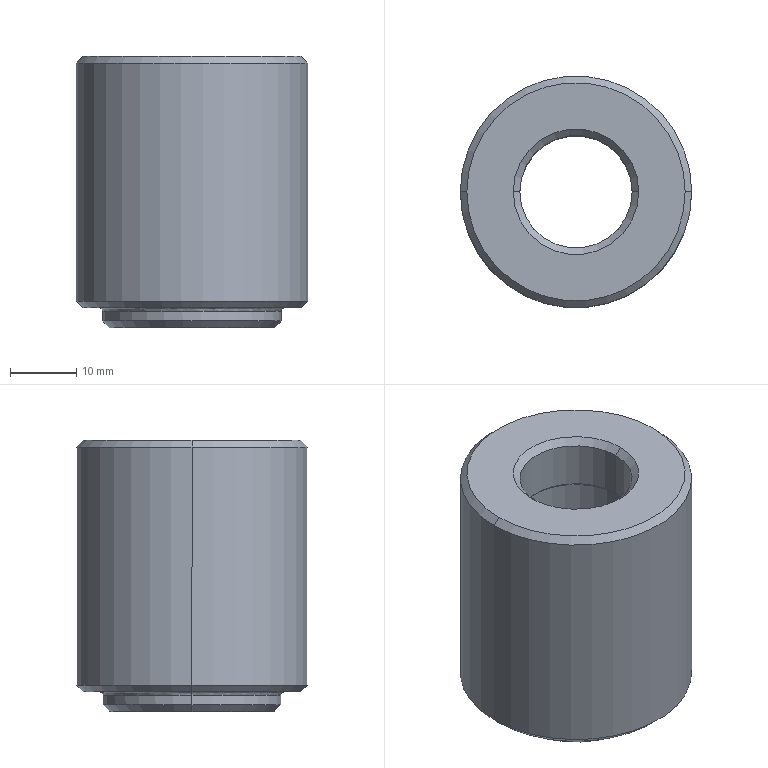Part | SolidWorks | features BaseBody 1 | 1 solid | 29 faces | box 35 x 35 x 41 mm | volume 28098 mm3 | cone 14 | cylinder 10 | plane 3 | spline 2 | commonest cylinder face diameters 17 x4 18 x2 27 x2 35 x2
STEP:
#1=CARTESIAN_POINT('',(-13.5,0.1036,-38.5));
#2=VERTEX_POINT('',#1);
#3=CARTESIAN_POINT('',(13.5,0.,-38.5));
#4=VERTEX_POINT('',#3);
#5=CARTESIAN_POINT('',(0.,0.,-38.5));
#6=DIRECTION('',(0.,0.,-1.));
#7=DIRECTION('',(1.,-0.007674,0.));
#8=AXIS2_PLACEMENT_3D('',#5,#6,#7);
#9=CIRCLE('',#8,13.5);
#10=EDGE_CURVE('',#2,#4,#9,.T.);
#11=ORIENTED_EDGE('',*,*,#10,.F.);
#12=CARTESIAN_POINT('',(-14.,0.1074,-38.));
#13=VERTEX_POINT('',#12);
#14=CARTESIAN_POINT('',(-14.,0.1074,-38.5));
#15=DIRECTION('',(-0.007674,-1.,0.));
#16=DIRECTION('',(-1.,0.007674,0.));
#17=AXIS2_PLACEMENT_3D('',#14,#15,#16);
#18=CIRCLE('',#17,0.5);
#19=EDGE_CURVE('',#2,#13,#18,.T.);
#20=ORIENTED_EDGE('',*,*,#19,.T.);
#21=CARTESIAN_POINT('',(14.,0.,-38.));
#22=VERTEX_POINT('',#21);
#23=CARTESIAN_POINT('',(-14.,0.1074,-38.));
#24=CARTESIAN_POINT('',(-13.786,27.893,-38.));
#25=CARTESIAN_POINT('',(14.,27.787,-38.));
#26=CARTESIAN_POINT('',(14.,0.,-38.));
#27=(BOUNDED_CURVE()B_SPLINE_CURVE(3,(#23,#24,#25,#26),.UNSPECIFIED.,.F.,.T.)B_SPLINE_CURVE_WITH_KNOTS((4,4),(0.002443,1.),.UNSPECIFIED.)CURVE()GEOMETRIC_REPRESENTATION_ITEM()RATIONAL_B_SPLINE_CURVE((1.,0.3359,0.3359,1.))REPRESENTATION_ITEM(''));
#28=EDGE_CURVE('',#13,#22,#27,.T.);
#29=ORIENTED_EDGE('',*,*,#28,.T.);
#30=CARTESIAN_POINT('',(14.,-0.1074,-38.));
#31=VERTEX_POINT('',#30);
#32=CARTESIAN_POINT('',(14.,0.,-38.));
#33=CARTESIAN_POINT('',(14.,-0.03581,-38.));
#34=CARTESIAN_POINT('',(14.,-0.07162,-38.));
#35=CARTESIAN_POINT('',(14.,-0.1074,-38.));
#36=(BOUNDED_CURVE()B_SPLINE_CURVE(3,(#32,#33,#34,#35),.UNSPECIFIED.,.F.,.F.)B_SPLINE_CURVE_WITH_KNOTS((4,4),(0.,0.002443),.UNSPECIFIED.)CURVE()GEOMETRIC_REPRESENTATION_ITEM()RATIONAL_B_SPLINE_CURVE((1.,1.,1.,1.))REPRESENTATION_ITEM(''));
#37=EDGE_CURVE('',#22,#31,#36,.T.);
#38=ORIENTED_EDGE('',*,*,#37,.T.);
#39=CARTESIAN_POINT('',(13.5,-0.1036,-38.5));
#40=VERTEX_POINT('',#39);
#41=CARTESIAN_POINT('',(14.,-0.1074,-38.5));
#42=DIRECTION('',(0.007674,1.,0.));
#43=DIRECTION('',(1.,-0.007674,0.));
#44=AXIS2_PLACEMENT_3D('',#41,#42,#43);
#45=CIRCLE('',#44,0.5);
#46=EDGE_CURVE('',#40,#31,#45,.T.);
#47=ORIENTED_EDGE('',*,*,#46,.F.);
#48=CARTESIAN_POINT('',(0.,0.,-38.5));
#49=DIRECTION('',(0.,0.,-1.));
#50=DIRECTION('',(1.,-0.007674,0.));
#51=AXIS2_PLACEMENT_3D('',#48,#49,#50);
#52=CIRCLE('',#51,13.5);
#53=EDGE_CURVE('',#4,#40,#52,.T.);
#54=ORIENTED_EDGE('',*,*,#53,.F.);
#55=EDGE_LOOP('',(#11,#20,#29,#38,#47,#54));
#56=FACE_OUTER_BOUND('',#55,.T.);
#57=CARTESIAN_POINT('',(13.5,-0.1036,-38.5));
#58=CARTESIAN_POINT('',(13.707,26.896,-38.5));
#59=CARTESIAN_POINT('',(-13.292,27.103,-38.5));
#60=CARTESIAN_POINT('',(-13.5,0.1036,-38.5));
#61=CARTESIAN_POINT('',(13.5,-0.1036,-38.207));
#62=CARTESIAN_POINT('',(13.707,26.896,-38.207));
#63=CARTESIAN_POINT('',(-13.292,27.103,-38.207));
#64=CARTESIAN_POINT('',(-13.5,0.1036,-38.207));
#65=CARTESIAN_POINT('',(13.707,-0.1052,-38.));
#66=CARTESIAN_POINT('',(13.917,27.308,-38.));
#67=CARTESIAN_POINT('',(-13.496,27.519,-38.));
#68=CARTESIAN_POINT('',(-13.707,0.1052,-38.));
#69=CARTESIAN_POINT('',(14.,-0.1074,-38.));
#70=CARTESIAN_POINT('',(14.214,27.892,-38.));
#71=CARTESIAN_POINT('',(-13.785,28.107,-38.));
#72=CARTESIAN_POINT('',(-14.,0.1074,-38.));
#73=(BOUNDED_SURFACE()B_SPLINE_SURFACE(3,3,((#57,#58,#59,#60),(#61,#62,#63,#64),(#65,#66,#67,#68),(#69,#70,#71,#72)),.UNSPECIFIED.,.F.,.F.,.F.)B_SPLINE_SURFACE_WITH_KNOTS((4,4),(4,4),(0.,1.),(0.,1.),.UNSPECIFIED.)GEOMETRIC_REPRESENTATION_ITEM()RATIONAL_B_SPLINE_SURFACE(((1.,0.3333,0.3333,1.),(0.8047,0.2682,0.2682,0.8047),(0.8047,0.2682,0.2682,0.8047),(1.,0.3333,0.3333,1.)))REPRESENTATION_ITEM('')SURFACE());
#74=ADVANCED_FACE('',(#56),#73,.F.);
#75=CARTESIAN_POINT('',(17.5,0.,-37.));
#76=VERTEX_POINT('',#75);
#77=CARTESIAN_POINT('',(-17.5,0.,-37.));
#78=VERTEX_POINT('',#77);
#79=CARTESIAN_POINT('',(0.,0.,-37.));
#80=DIRECTION('',(0.,0.,1.));
#81=DIRECTION('',(1.,0.,0.));
#82=AXIS2_PLACEMENT_3D('',#79,#80,#81);
#83=CIRCLE('',#82,17.5);
#84=EDGE_CURVE('',#76,#78,#83,.T.);
#85=ORIENTED_EDGE('',*,*,#84,.T.);
#86=CARTESIAN_POINT('',(-17.5,0.,-1.));
#87=VERTEX_POINT('',#86);
#88=CARTESIAN_POINT('',(-17.5,0.,-43.05));
#89=DIRECTION('',(0.,0.,1.));
#90=VECTOR('',#89,1000.);
#91=LINE('',#88,#90);
#92=EDGE_CURVE('',#78,#87,#91,.T.);
#93=ORIENTED_EDGE('',*,*,#92,.T.);
#94=CARTESIAN_POINT('',(17.5,0.,-1.));
#95=VERTEX_POINT('',#94);
#96=CARTESIAN_POINT('',(0.,0.,-1.));
#97=DIRECTION('',(0.,0.,-1.));
#98=DIRECTION('',(1.,0.,0.));
#99=AXIS2_PLACEMENT_3D('',#96,#97,#98);
#100=CIRCLE('',#99,17.5);
#101=EDGE_CURVE('',#87,#95,#100,.T.);
#102=ORIENTED_EDGE('',*,*,#101,.T.);
#103=CARTESIAN_POINT('',(17.5,0.,-43.05));
#104=DIRECTION('',(0.,0.,1.));
#105=VECTOR('',#104,1000.);
#106=LINE('',#103,#105);
#107=EDGE_CURVE('',#76,#95,#106,.T.);
#108=ORIENTED_EDGE('',*,*,#107,.F.);
#109=EDGE_LOOP('',(#85,#93,#102,#108));
#110=FACE_OUTER_BOUND('',#109,.T.);
#111=CARTESIAN_POINT('',(0.,0.,-43.05));
#112=DIRECTION('',(0.,0.,1.));
#113=DIRECTION('',(1.,0.,0.));
#114=AXIS2_PLACEMENT_3D('',#111,#112,#113);
#115=CYLINDRICAL_SURFACE('',#114,17.5);
#116=ADVANCED_FACE('',(#110),#115,.T.);
#117=CARTESIAN_POINT('',(16.5,0.,-38.));
#118=VERTEX_POINT('',#117);
#119=CARTESIAN_POINT('',(-16.5,0.,-38.));
#120=VERTEX_POINT('',#119);
#121=CARTESIAN_POINT('',(0.,0.,-38.));
#122=DIRECTION('',(0.,0.,1.));
#123=DIRECTION('',(1.,0.,0.));
#124=AXIS2_PLACEMENT_3D('',#121,#122,#123);
#125=CIRCLE('',#124,16.5);
#126=EDGE_CURVE('',#118,#120,#125,.T.);
#127=ORIENTED_EDGE('',*,*,#126,.T.);
#128=CARTESIAN_POINT('',(-17.5,0.,-37.));
#129=DIRECTION('',(-0.7071,0.,0.7071));
#130=VECTOR('',#129,1000.);
#131=LINE('',#128,#130);
#132=EDGE_CURVE('',#120,#78,#131,.T.);
#133=ORIENTED_EDGE('',*,*,#132,.T.);
#134=ORIENTED_EDGE('',*,*,#84,.F.);
#135=CARTESIAN_POINT('',(17.5,0.,-37.));
#136=DIRECTION('',(0.7071,0.,0.7071));
#137=VECTOR('',#136,1000.);
#138=LINE('',#135,#137);
#139=EDGE_CURVE('',#118,#76,#138,.T.);
#140=ORIENTED_EDGE('',*,*,#139,.F.);
#141=EDGE_LOOP('',(#127,#133,#134,#140));
#142=FACE_OUTER_BOUND('',#141,.T.);
#143=CARTESIAN_POINT('',(0.,0.,-37.));
#144=DIRECTION('',(0.,0.,1.));
#145=DIRECTION('',(1.,0.,0.));
#146=AXIS2_PLACEMENT_3D('',#143,#144,#145);
#147=CONICAL_SURFACE('',#146,17.5,0.7854);
#148=ADVANCED_FACE('',(#142),#147,.T.);
#149=CARTESIAN_POINT('',(-16.5,0.,0.));
#150=VERTEX_POINT('',#149);
#151=CARTESIAN_POINT('',(16.5,0.,0.));
#152=VERTEX_POINT('',#151);
#153=CARTESIAN_POINT('',(0.,0.,0.));
#154=DIRECTION('',(0.,0.,-1.));
#155=DIRECTION('',(-1.,0.,0.));
#156=AXIS2_PLACEMENT_3D('',#153,#154,#155);
#157=CIRCLE('',#156,16.5);
#158=EDGE_CURVE('',#150,#152,#157,.T.);
#159=ORIENTED_EDGE('',*,*,#158,.T.);
#160=CARTESIAN_POINT('',(17.5,0.,-1.));
#161=DIRECTION('',(0.7071,0.,-0.7071));
#162=VECTOR('',#161,1000.);
#163=LINE('',#160,#162);
#164=EDGE_CURVE('',#152,#95,#163,.T.);
#165=ORIENTED_EDGE('',*,*,#164,.T.);
#166=ORIENTED_EDGE('',*,*,#101,.F.);
#167=CARTESIAN_POINT('',(-17.5,0.,-1.));
#168=DIRECTION('',(-0.7071,0.,-0.7071));
#169=VECTOR('',#168,1000.);
#170=LINE('',#167,#169);
#171=EDGE_CURVE('',#150,#87,#170,.T.);
#172=ORIENTED_EDGE('',*,*,#171,.F.);
#173=EDGE_LOOP('',(#159,#165,#166,#172));
#174=FACE_OUTER_BOUND('',#173,.T.);
#175=CARTESIAN_POINT('',(0.,0.,-1.));
#176=DIRECTION('',(0.,0.,-1.));
#177=DIRECTION('',(-1.,0.,0.));
#178=AXIS2_PLACEMENT_3D('',#175,#176,#177);
#179=CONICAL_SURFACE('',#178,17.5,0.7854);
#180=ADVANCED_FACE('',(#174),#179,.T.);
#181=CARTESIAN_POINT('',(-8.5,0.,-1.));
#182=VERTEX_POINT('',#181);
#183=CARTESIAN_POINT('',(8.5,0.,-1.));
#184=VERTEX_POINT('',#183);
#185=CARTESIAN_POINT('',(0.,0.,-1.));
#186=DIRECTION('',(0.,0.,1.));
#187=DIRECTION('',(0.,-1.,0.));
#188=AXIS2_PLACEMENT_3D('',#185,#186,#187);
#189=CIRCLE('',#188,8.5);
#190=EDGE_CURVE('',#182,#184,#189,.T.);
#191=ORIENTED_EDGE('',*,*,#190,.F.);
#192=CARTESIAN_POINT('',(-9.5,0.,0.));
#193=VERTEX_POINT('',#192);
#194=CARTESIAN_POINT('',(-9.5,0.,0.));
#195=DIRECTION('',(-0.7071,0.,0.7071));
#196=VECTOR('',#195,1000.);
#197=LINE('',#194,#196);
#198=EDGE_CURVE('',#182,#193,#197,.T.);
#199=ORIENTED_EDGE('',*,*,#198,.T.);
#200=CARTESIAN_POINT('',(9.5,0.,0.));
#201=VERTEX_POINT('',#200);
#202=CARTESIAN_POINT('',(0.,0.,0.));
#203=DIRECTION('',(0.,0.,-1.));
#204=DIRECTION('',(1.,0.,0.));
#205=AXIS2_PLACEMENT_3D('',#202,#203,#204);
#206=CIRCLE('',#205,9.5);
#207=EDGE_CURVE('',#201,#193,#206,.T.);
#208=ORIENTED_EDGE('',*,*,#207,.F.);
#209=CARTESIAN_POINT('',(9.5,0.,0.));
#210=DIRECTION('',(0.7071,0.,0.7071));
#211=VECTOR('',#210,1000.);
#212=LINE('',#209,#211);
#213=EDGE_CURVE('',#184,#201,#212,.T.);
#214=ORIENTED_EDGE('',*,*,#213,.F.);
#215=EDGE_LOOP('',(#191,#199,#208,#214));
#216=FACE_OUTER_BOUND('',#215,.T.);
#217=CARTESIAN_POINT('',(0.,0.,0.));
#218=DIRECTION('',(0.,0.,1.));
#219=DIRECTION('',(1.,0.,0.));
#220=AXIS2_PLACEMENT_3D('',#217,#218,#219);
#221=CONICAL_SURFACE('',#220,9.5,0.7854);
#222=ADVANCED_FACE('',(#216),#221,.F.);
#223=CARTESIAN_POINT('',(13.5,0.,-40.));
#224=VERTEX_POINT('',#223);
#225=CARTESIAN_POINT('',(-13.5,0.,-40.));
#226=VERTEX_POINT('',#225);
#227=CARTESIAN_POINT('',(0.,0.,-40.));
#228=DIRECTION('',(0.,0.,1.));
#229=DIRECTION('',(1.,0.,0.));
#230=AXIS2_PLACEMENT_3D('',#227,#228,#229);
#231=CIRCLE('',#230,13.5);
#232=EDGE_CURVE('',#224,#226,#231,.T.);
#233=ORIENTED_EDGE('',*,*,#232,.T.);
#234=CARTESIAN_POINT('',(-13.5,0.,-38.5));
#235=VERTEX_POINT('',#234);
#236=CARTESIAN_POINT('',(-13.5,0.,-43.05));
#237=DIRECTION('',(0.,0.,1.));
#238=VECTOR('',#237,1000.);
#239=LINE('',#236,#238);
#240=EDGE_CURVE('',#226,#235,#239,.T.);
#241=ORIENTED_EDGE('',*,*,#240,.T.);
#242=CARTESIAN_POINT('',(0.,0.,-38.5));
#243=DIRECTION('',(0.,0.,-1.));
#244=DIRECTION('',(1.,-0.007674,0.));
#245=AXIS2_PLACEMENT_3D('',#242,#243,#244);
#246=CIRCLE('',#245,13.5);
#247=EDGE_CURVE('',#235,#2,#246,.T.);
#248=ORIENTED_EDGE('',*,*,#247,.T.);
#249=ORIENTED_EDGE('',*,*,#10,.T.);
#250=CARTESIAN_POINT('',(13.5,0.,-43.05));
#251=DIRECTION('',(0.,0.,1.));
#252=VECTOR('',#251,1000.);
#253=LINE('',#250,#252);
#254=EDGE_CURVE('',#224,#4,#253,.T.);
#255=ORIENTED_EDGE('',*,*,#254,.F.);
#256=EDGE_LOOP('',(#233,#241,#248,#249,#255));
#257=FACE_OUTER_BOUND('',#256,.T.);
#258=CARTESIAN_POINT('',(0.,0.,-43.05));
#259=DIRECTION('',(0.,0.,1.));
#260=DIRECTION('',(1.,0.,0.));
#261=AXIS2_PLACEMENT_3D('',#258,#259,#260);
#262=CYLINDRICAL_SURFACE('',#261,13.5);
#263=ADVANCED_FACE('',(#257),#262,.T.);
#264=CARTESIAN_POINT('',(-8.5,0.,-8.));
#265=VERTEX_POINT('',#264);
#266=CARTESIAN_POINT('',(8.5,0.,-8.));
#267=VERTEX_POINT('',#266);
#268=CARTESIAN_POINT('',(0.,0.,-8.));
#269=DIRECTION('',(0.,0.,1.));
#270=DIRECTION('',(1.,0.,0.));
#271=AXIS2_PLACEMENT_3D('',#268,#269,#270);
#272=CIRCLE('',#271,8.5);
#273=EDGE_CURVE('',#265,#267,#272,.T.);
#274=ORIENTED_EDGE('',*,*,#273,.F.);
#275=CARTESIAN_POINT('',(-8.5,0.,-43.05));
#276=DIRECTION('',(0.,0.,1.));
#277=VECTOR('',#276,1000.);
#278=LINE('',#275,#277);
#279=EDGE_CURVE('',#265,#182,#278,.T.);
#280=ORIENTED_EDGE('',*,*,#279,.T.);
#281=ORIENTED_EDGE('',*,*,#190,.T.);
#282=CARTESIAN_POINT('',(8.5,0.,-43.05));
#283=DIRECTION('',(0.,0.,1.));
#284=VECTOR('',#283,1000.);
#285=LINE('',#282,#284);
#286=EDGE_CURVE('',#267,#184,#285,.T.);
#287=ORIENTED_EDGE('',*,*,#286,.F.);
#288=EDGE_LOOP('',(#274,#280,#281,#287));
#289=FACE_OUTER_BOUND('',#288,.T.);
#290=CARTESIAN_POINT('',(0.,0.,-43.05));
#291=DIRECTION('',(0.,0.,1.));
#292=DIRECTION('',(1.,0.,0.));
#293=AXIS2_PLACEMENT_3D('',#290,#291,#292);
#294=CYLINDRICAL_SURFACE('',#293,8.5);
#295=ADVANCED_FACE('',(#289),#294,.F.);
#296=CARTESIAN_POINT('',(12.5,0.,-41.));
#297=VERTEX_POINT('',#296);
#298=CARTESIAN_POINT('',(-12.5,0.,-41.));
#299=VERTEX_POINT('',#298);
#300=CARTESIAN_POINT('',(0.,0.,-41.));
#301=DIRECTION('',(0.,0.,1.));
#302=DIRECTION('',(1.,0.,0.));
#303=AXIS2_PLACEMENT_3D('',#300,#301,#302);
#304=CIRCLE('',#303,12.5);
#305=EDGE_CURVE('',#297,#299,#304,.T.);
#306=ORIENTED_EDGE('',*,*,#305,.T.);
#307=CARTESIAN_POINT('',(-13.5,0.,-40.));
#308=DIRECTION('',(-0.7071,0.,0.7071));
#309=VECTOR('',#308,1000.);
#310=LINE('',#307,#309);
#311=EDGE_CURVE('',#299,#226,#310,.T.);
#312=ORIENTED_EDGE('',*,*,#311,.T.);
#313=ORIENTED_EDGE('',*,*,#232,.F.);
#314=CARTESIAN_POINT('',(13.5,0.,-40.));
#315=DIRECTION('',(0.7071,0.,0.7071));
#316=VECTOR('',#315,1000.);
#317=LINE('',#314,#316);
#318=EDGE_CURVE('',#297,#224,#317,.T.);
#319=ORIENTED_EDGE('',*,*,#318,.F.);
#320=EDGE_LOOP('',(#306,#312,#313,#319));
#321=FACE_OUTER_BOUND('',#320,.T.);
#322=CARTESIAN_POINT('',(0.,0.,-40.));
#323=DIRECTION('',(0.,0.,1.));
#324=DIRECTION('',(1.,0.,0.));
#325=AXIS2_PLACEMENT_3D('',#322,#323,#324);
#326=CONICAL_SURFACE('',#325,13.5,0.7854);
#327=ADVANCED_FACE('',(#321),#326,.T.);
#328=ORIENTED_EDGE('',*,*,#273,.T.);
#329=CARTESIAN_POINT('',(9.,0.,-8.5));
#330=VERTEX_POINT('',#329);
#331=CARTESIAN_POINT('',(9.,0.,-8.5));
#332=DIRECTION('',(0.7071,0.,-0.7071));
#333=VECTOR('',#332,1000.);
#334=LINE('',#331,#333);
#335=EDGE_CURVE('',#267,#330,#334,.T.);
#336=ORIENTED_EDGE('',*,*,#335,.T.);
#337=CARTESIAN_POINT('',(-9.,0.,-8.5));
#338=VERTEX_POINT('',#337);
#339=CARTESIAN_POINT('',(0.,0.,-8.5));
#340=DIRECTION('',(0.,0.,1.));
#341=DIRECTION('',(1.,0.,0.));
#342=AXIS2_PLACEMENT_3D('',#339,#340,#341);
#343=CIRCLE('',#342,9.);
#344=EDGE_CURVE('',#338,#330,#343,.T.);
#345=ORIENTED_EDGE('',*,*,#344,.F.);
#346=CARTESIAN_POINT('',(-9.,0.,-8.5));
#347=DIRECTION('',(-0.7071,0.,-0.7071));
#348=VECTOR('',#347,1000.);
#349=LINE('',#346,#348);
#350=EDGE_CURVE('',#265,#338,#349,.T.);
#351=ORIENTED_EDGE('',*,*,#350,.F.);
#352=EDGE_LOOP('',(#328,#336,#345,#351));
#353=FACE_OUTER_BOUND('',#352,.T.);
#354=CARTESIAN_POINT('',(0.,0.,-8.5));
#355=DIRECTION('',(0.,0.,-1.));
#356=DIRECTION('',(-1.,0.,0.));
#357=AXIS2_PLACEMENT_3D('',#354,#355,#356);
#358=CONICAL_SURFACE('',#357,9.,0.7854);
#359=ADVANCED_FACE('',(#353),#358,.F.);
#360=CARTESIAN_POINT('',(-9.,0.,-32.5));
#361=VERTEX_POINT('',#360);
#362=CARTESIAN_POINT('',(9.,0.,-32.5));
#363=VERTEX_POINT('',#362);
#364=CARTESIAN_POINT('',(0.,0.,-32.5));
#365=DIRECTION('',(0.,0.,1.));
#366=DIRECTION('',(1.,0.,0.));
#367=AXIS2_PLACEMENT_3D('',#364,#365,#366);
#368=CIRCLE('',#367,9.);
#369=EDGE_CURVE('',#361,#363,#368,.T.);
#370=ORIENTED_EDGE('',*,*,#369,.F.);
#371=CARTESIAN_POINT('',(-9.,0.,-43.05));
#372=DIRECTION('',(0.,0.,1.));
#373=VECTOR('',#372,1000.);
#374=LINE('',#371,#373);
#375=EDGE_CURVE('',#361,#338,#374,.T.);
#376=ORIENTED_EDGE('',*,*,#375,.T.);
#377=ORIENTED_EDGE('',*,*,#344,.T.);
#378=CARTESIAN_POINT('',(9.,0.,-43.05));
#379=DIRECTION('',(0.,0.,1.));
#380=VECTOR('',#379,1000.);
#381=LINE('',#378,#380);
#382=EDGE_CURVE('',#363,#330,#381,.T.);
#383=ORIENTED_EDGE('',*,*,#382,.F.);
#384=EDGE_LOOP('',(#370,#376,#377,#383));
#385=FACE_OUTER_BOUND('',#384,.T.);
#386=CARTESIAN_POINT('',(0.,0.,-43.05));
#387=DIRECTION('',(0.,0.,1.));
#388=DIRECTION('',(1.,0.,0.));
#389=AXIS2_PLACEMENT_3D('',#386,#387,#388);
#390=CYLINDRICAL_SURFACE('',#389,9.);
#391=ADVANCED_FACE('',(#385),#390,.F.);
#392=CARTESIAN_POINT('',(8.5,0.,-40.));
#393=VERTEX_POINT('',#392);
#394=CARTESIAN_POINT('',(-8.5,0.,-40.));
#395=VERTEX_POINT('',#394);
#396=CARTESIAN_POINT('',(0.,0.,-40.));
#397=DIRECTION('',(0.,0.,-1.));
#398=DIRECTION('',(0.,-1.,0.));
#399=AXIS2_PLACEMENT_3D('',#396,#397,#398);
#400=CIRCLE('',#399,8.5);
#401=EDGE_CURVE('',#393,#395,#400,.T.);
#402=ORIENTED_EDGE('',*,*,#401,.F.);
#403=CARTESIAN_POINT('',(9.5,0.,-41.));
#404=VERTEX_POINT('',#403);
#405=CARTESIAN_POINT('',(9.5,0.,-41.));
#406=DIRECTION('',(0.7071,0.,-0.7071));
#407=VECTOR('',#406,1000.);
#408=LINE('',#405,#407);
#409=EDGE_CURVE('',#393,#404,#408,.T.);
#410=ORIENTED_EDGE('',*,*,#409,.T.);
#411=CARTESIAN_POINT('',(-9.5,0.,-41.));
#412=VERTEX_POINT('',#411);
#413=CARTESIAN_POINT('',(0.,0.,-41.));
#414=DIRECTION('',(0.,0.,-1.));
#415=DIRECTION('',(-1.,0.,0.));
#416=AXIS2_PLACEMENT_3D('',#413,#414,#415);
#417=CIRCLE('',#416,9.5);
#418=EDGE_CURVE('',#404,#412,#417,.T.);
#419=ORIENTED_EDGE('',*,*,#418,.T.);
#420=CARTESIAN_POINT('',(-9.5,0.,-41.));
#421=DIRECTION('',(-0.7071,0.,-0.7071));
#422=VECTOR('',#421,1000.);
#423=LINE('',#420,#422);
#424=EDGE_CURVE('',#395,#412,#423,.T.);
#425=ORIENTED_EDGE('',*,*,#424,.F.);
#426=EDGE_LOOP('',(#402,#410,#419,#425));
#427=FACE_OUTER_BOUND('',#426,.T.);
#428=CARTESIAN_POINT('',(0.,0.,-41.));
#429=DIRECTION('',(0.,0.,-1.));
#430=DIRECTION('',(-1.,0.,0.));
#431=AXIS2_PLACEMENT_3D('',#428,#429,#430);
#432=CONICAL_SURFACE('',#431,9.5,0.7854);
#433=ADVANCED_FACE('',(#427),#432,.F.);
#434=CARTESIAN_POINT('',(-8.5,0.,-33.));
#435=VERTEX_POINT('',#434);
#436=CARTESIAN_POINT('',(8.5,0.,-33.));
#437=VERTEX_POINT('',#436);
#438=CARTESIAN_POINT('',(0.,0.,-33.));
#439=DIRECTION('',(0.,0.,1.));
#440=DIRECTION('',(-1.,0.,0.));
#441=AXIS2_PLACEMENT_3D('',#438,#439,#440);
#442=CIRCLE('',#441,8.5);
#443=EDGE_CURVE('',#435,#437,#442,.T.);
#444=ORIENTED_EDGE('',*,*,#443,.F.);
#445=CARTESIAN_POINT('',(-9.,0.,-32.5));
#446=DIRECTION('',(-0.7071,0.,0.7071));
#447=VECTOR('',#446,1000.);
#448=LINE('',#445,#447);
#449=EDGE_CURVE('',#435,#361,#448,.T.);
#450=ORIENTED_EDGE('',*,*,#449,.T.);
#451=ORIENTED_EDGE('',*,*,#369,.T.);
#452=CARTESIAN_POINT('',(9.,0.,-32.5));
#453=DIRECTION('',(0.7071,0.,0.7071));
#454=VECTOR('',#453,1000.);
#455=LINE('',#452,#454);
#456=EDGE_CURVE('',#437,#363,#455,.T.);
#457=ORIENTED_EDGE('',*,*,#456,.F.);
#458=EDGE_LOOP('',(#444,#450,#451,#457));
#459=FACE_OUTER_BOUND('',#458,.T.);
#460=CARTESIAN_POINT('',(0.,0.,-32.5));
#461=DIRECTION('',(0.,0.,1.));
#462=DIRECTION('',(1.,0.,0.));
#463=AXIS2_PLACEMENT_3D('',#460,#461,#462);
#464=CONICAL_SURFACE('',#463,9.,0.7854);
#465=ADVANCED_FACE('',(#459),#464,.F.);
#466=ORIENTED_EDGE('',*,*,#401,.T.);
#467=CARTESIAN_POINT('',(-8.5,0.,-43.05));
#468=DIRECTION('',(0.,0.,1.));
#469=VECTOR('',#468,1000.);
#470=LINE('',#467,#469);
#471=EDGE_CURVE('',#395,#435,#470,.T.);
#472=ORIENTED_EDGE('',*,*,#471,.T.);
#473=ORIENTED_EDGE('',*,*,#443,.T.);
#474=CARTESIAN_POINT('',(8.5,0.,-43.05));
#475=DIRECTION('',(0.,0.,1.));
#476=VECTOR('',#475,1000.);
#477=LINE('',#474,#476);
#478=EDGE_CURVE('',#393,#437,#477,.T.);
#479=ORIENTED_EDGE('',*,*,#478,.F.);
#480=EDGE_LOOP('',(#466,#472,#473,#479));
#481=FACE_OUTER_BOUND('',#480,.T.);
#482=CARTESIAN_POINT('',(0.,0.,-43.05));
#483=DIRECTION('',(0.,0.,1.));
#484=DIRECTION('',(1.,0.,0.));
#485=AXIS2_PLACEMENT_3D('',#482,#483,#484);
#486=CYLINDRICAL_SURFACE('',#485,8.5);
#487=ADVANCED_FACE('',(#481),#486,.F.);
#488=ORIENTED_EDGE('',*,*,#92,.F.);
#489=CARTESIAN_POINT('',(0.,0.,-37.));
#490=DIRECTION('',(0.,0.,1.));
#491=DIRECTION('',(1.,0.,0.));
#492=AXIS2_PLACEMENT_3D('',#489,#490,#491);
#493=CIRCLE('',#492,17.5);
#494=EDGE_CURVE('',#78,#76,#493,.T.);
#495=ORIENTED_EDGE('',*,*,#494,.T.);
#496=ORIENTED_EDGE('',*,*,#107,.T.);
#497=CARTESIAN_POINT('',(0.,0.,-1.));
#498=DIRECTION('',(0.,0.,-1.));
#499=DIRECTION('',(1.,0.,0.));
#500=AXIS2_PLACEMENT_3D('',#497,#498,#499);
#501=CIRCLE('',#500,17.5);
#502=EDGE_CURVE('',#95,#87,#501,.T.);
#503=ORIENTED_EDGE('',*,*,#502,.T.);
#504=EDGE_LOOP('',(#488,#495,#496,#503));
#505=FACE_OUTER_BOUND('',#504,.T.);
#506=CARTESIAN_POINT('',(0.,0.,-43.05));
#507=DIRECTION('',(0.,0.,1.));
#508=DIRECTION('',(1.,0.,0.));
#509=AXIS2_PLACEMENT_3D('',#506,#507,#508);
#510=CYLINDRICAL_SURFACE('',#509,17.5);
#511=ADVANCED_FACE('',(#505),#510,.T.);
#512=ORIENTED_EDGE('',*,*,#132,.F.);
#513=CARTESIAN_POINT('',(0.,0.,-38.));
#514=DIRECTION('',(0.,0.,1.));
#515=DIRECTION('',(1.,0.,0.));
#516=AXIS2_PLACEMENT_3D('',#513,#514,#515);
#517=CIRCLE('',#516,16.5);
#518=EDGE_CURVE('',#120,#118,#517,.T.);
#519=ORIENTED_EDGE('',*,*,#518,.T.);
#520=ORIENTED_EDGE('',*,*,#139,.T.);
#521=ORIENTED_EDGE('',*,*,#494,.F.);
#522=EDGE_LOOP('',(#512,#519,#520,#521));
#523=FACE_OUTER_BOUND('',#522,.T.);
#524=CARTESIAN_POINT('',(0.,0.,-37.));
#525=DIRECTION('',(0.,0.,1.));
#526=DIRECTION('',(1.,0.,0.));
#527=AXIS2_PLACEMENT_3D('',#524,#525,#526);
#528=CONICAL_SURFACE('',#527,17.5,0.7854);
#529=ADVANCED_FACE('',(#523),#528,.T.);
#530=ORIENTED_EDGE('',*,*,#164,.F.);
#531=CARTESIAN_POINT('',(0.,0.,0.));
#532=DIRECTION('',(0.,0.,-1.));
#533=DIRECTION('',(-1.,0.,0.));
#534=AXIS2_PLACEMENT_3D('',#531,#532,#533);
#535=CIRCLE('',#534,16.5);
#536=EDGE_CURVE('',#152,#150,#535,.T.);
#537=ORIENTED_EDGE('',*,*,#536,.T.);
#538=ORIENTED_EDGE('',*,*,#171,.T.);
#539=ORIENTED_EDGE('',*,*,#502,.F.);
#540=EDGE_LOOP('',(#530,#537,#538,#539));
#541=FACE_OUTER_BOUND('',#540,.T.);
#542=CARTESIAN_POINT('',(0.,0.,-1.));
#543=DIRECTION('',(0.,0.,-1.));
#544=DIRECTION('',(-1.,0.,0.));
#545=AXIS2_PLACEMENT_3D('',#542,#543,#544);
#546=CONICAL_SURFACE('',#545,17.5,0.7854);
#547=ADVANCED_FACE('',(#541),#546,.T.);
#548=ORIENTED_EDGE('',*,*,#37,.F.);
#549=ORIENTED_EDGE('',*,*,#28,.F.);
#550=CARTESIAN_POINT('',(-14.,0.,-38.));
#551=VERTEX_POINT('',#550);
#552=CARTESIAN_POINT('',(-14.,0.,-38.));
#553=CARTESIAN_POINT('',(-14.,0.03581,-38.));
#554=CARTESIAN_POINT('',(-14.,0.07162,-38.));
#555=CARTESIAN_POINT('',(-14.,0.1074,-38.));
#556=(BOUNDED_CURVE()B_SPLINE_CURVE(3,(#552,#553,#554,#555),.UNSPECIFIED.,.F.,.T.)B_SPLINE_CURVE_WITH_KNOTS((4,4),(0.,0.002443),.UNSPECIFIED.)CURVE()GEOMETRIC_REPRESENTATION_ITEM()RATIONAL_B_SPLINE_CURVE((1.,1.,1.,1.))REPRESENTATION_ITEM(''));
#557=EDGE_CURVE('',#551,#13,#556,.T.);
#558=ORIENTED_EDGE('',*,*,#557,.F.);
#559=CARTESIAN_POINT('',(14.,-0.1074,-38.));
#560=CARTESIAN_POINT('',(13.786,-27.893,-38.));
#561=CARTESIAN_POINT('',(-14.,-27.787,-38.));
#562=CARTESIAN_POINT('',(-14.,0.,-38.));
#563=(BOUNDED_CURVE()B_SPLINE_CURVE(3,(#559,#560,#561,#562),.UNSPECIFIED.,.F.,.F.)B_SPLINE_CURVE_WITH_KNOTS((4,4),(0.002443,1.),.UNSPECIFIED.)CURVE()GEOMETRIC_REPRESENTATION_ITEM()RATIONAL_B_SPLINE_CURVE((1.,0.3359,0.3359,1.))REPRESENTATION_ITEM(''));
#564=EDGE_CURVE('',#31,#551,#563,.T.);
#565=ORIENTED_EDGE('',*,*,#564,.F.);
#566=EDGE_LOOP('',(#548,#549,#558,#565));
#567=FACE_BOUND('',#566,.T.);
#568=ORIENTED_EDGE('',*,*,#126,.F.);
#569=ORIENTED_EDGE('',*,*,#518,.F.);
#570=EDGE_LOOP('',(#568,#569));
#571=FACE_OUTER_BOUND('',#570,.T.);
#572=CARTESIAN_POINT('',(0.,0.,-38.));
#573=DIRECTION('',(0.,0.,1.));
#574=DIRECTION('',(1.,0.,0.));
#575=AXIS2_PLACEMENT_3D('',#572,#573,#574);
#576=PLANE('',#575);
#577=ADVANCED_FACE('',(#567,#571),#576,.F.);
#578=ORIENTED_EDGE('',*,*,#207,.T.);
#579=CARTESIAN_POINT('',(0.,0.,0.));
#580=DIRECTION('',(0.,0.,-1.));
#581=DIRECTION('',(1.,0.,0.));
#582=AXIS2_PLACEMENT_3D('',#579,#580,#581);
#583=CIRCLE('',#582,9.5);
#584=EDGE_CURVE('',#193,#201,#583,.T.);
#585=ORIENTED_EDGE('',*,*,#584,.T.);
#586=EDGE_LOOP('',(#578,#585));
#587=FACE_BOUND('',#586,.T.);
#588=ORIENTED_EDGE('',*,*,#158,.F.);
#589=ORIENTED_EDGE('',*,*,#536,.F.);
#590=EDGE_LOOP('',(#588,#589));
#591=FACE_OUTER_BOUND('',#590,.T.);
#592=CARTESIAN_POINT('',(0.,0.,0.));
#593=DIRECTION('',(0.,0.,1.));
#594=DIRECTION('',(1.,0.,0.));
#595=AXIS2_PLACEMENT_3D('',#592,#593,#594);
#596=PLANE('',#595);
#597=ADVANCED_FACE('',(#587,#591),#596,.T.);
#598=ORIENTED_EDGE('',*,*,#19,.F.);
#599=ORIENTED_EDGE('',*,*,#247,.F.);
#600=CARTESIAN_POINT('',(0.,0.,-38.5));
#601=DIRECTION('',(0.,0.,-1.));
#602=DIRECTION('',(1.,-0.007674,0.));
#603=AXIS2_PLACEMENT_3D('',#600,#601,#602);
#604=CIRCLE('',#603,13.5);
#605=EDGE_CURVE('',#40,#235,#604,.T.);
#606=ORIENTED_EDGE('',*,*,#605,.F.);
#607=ORIENTED_EDGE('',*,*,#46,.T.);
#608=ORIENTED_EDGE('',*,*,#564,.T.);
#609=ORIENTED_EDGE('',*,*,#557,.T.);
#610=EDGE_LOOP('',(#598,#599,#606,#607,#608,#609));
#611=FACE_OUTER_BOUND('',#610,.T.);
#612=CARTESIAN_POINT('',(-13.5,0.1036,-38.5));
#613=CARTESIAN_POINT('',(-13.707,-26.896,-38.5));
#614=CARTESIAN_POINT('',(13.292,-27.103,-38.5));
#615=CARTESIAN_POINT('',(13.5,-0.1036,-38.5));
#616=CARTESIAN_POINT('',(-13.5,0.1036,-38.207));
#617=CARTESIAN_POINT('',(-13.707,-26.896,-38.207));
#618=CARTESIAN_POINT('',(13.292,-27.103,-38.207));
#619=CARTESIAN_POINT('',(13.5,-0.1036,-38.207));
#620=CARTESIAN_POINT('',(-13.707,0.1052,-38.));
#621=CARTESIAN_POINT('',(-13.917,-27.308,-38.));
#622=CARTESIAN_POINT('',(13.496,-27.519,-38.));
#623=CARTESIAN_POINT('',(13.707,-0.1052,-38.));
#624=CARTESIAN_POINT('',(-14.,0.1074,-38.));
#625=CARTESIAN_POINT('',(-14.214,-27.892,-38.));
#626=CARTESIAN_POINT('',(13.785,-28.107,-38.));
#627=CARTESIAN_POINT('',(14.,-0.1074,-38.));
#628=(BOUNDED_SURFACE()B_SPLINE_SURFACE(3,3,((#612,#613,#614,#615),(#616,#617,#618,#619),(#620,#621,#622,#623),(#624,#625,#626,#627)),.UNSPECIFIED.,.F.,.F.,.F.)B_SPLINE_SURFACE_WITH_KNOTS((4,4),(4,4),(0.,1.),(0.,1.),.UNSPECIFIED.)GEOMETRIC_REPRESENTATION_ITEM()RATIONAL_B_SPLINE_SURFACE(((1.,0.3333,0.3333,1.),(0.8047,0.2682,0.2682,0.8047),(0.8047,0.2682,0.2682,0.8047),(1.,0.3333,0.3333,1.)))REPRESENTATION_ITEM('')SURFACE());
#629=ADVANCED_FACE('',(#611),#628,.F.);
#630=ORIENTED_EDGE('',*,*,#198,.F.);
#631=CARTESIAN_POINT('',(0.,0.,-1.));
#632=DIRECTION('',(0.,0.,1.));
#633=DIRECTION('',(0.,-1.,0.));
#634=AXIS2_PLACEMENT_3D('',#631,#632,#633);
#635=CIRCLE('',#634,8.5);
#636=EDGE_CURVE('',#184,#182,#635,.T.);
#637=ORIENTED_EDGE('',*,*,#636,.F.);
#638=ORIENTED_EDGE('',*,*,#213,.T.);
#639=ORIENTED_EDGE('',*,*,#584,.F.);
#640=EDGE_LOOP('',(#630,#637,#638,#639));
#641=FACE_OUTER_BOUND('',#640,.T.);
#642=CARTESIAN_POINT('',(0.,0.,0.));
#643=DIRECTION('',(0.,0.,1.));
#644=DIRECTION('',(1.,0.,0.));
#645=AXIS2_PLACEMENT_3D('',#642,#643,#644);
#646=CONICAL_SURFACE('',#645,9.5,0.7854);
#647=ADVANCED_FACE('',(#641),#646,.F.);
#648=ORIENTED_EDGE('',*,*,#240,.F.);
#649=CARTESIAN_POINT('',(0.,0.,-40.));
#650=DIRECTION('',(0.,0.,1.));
#651=DIRECTION('',(1.,0.,0.));
#652=AXIS2_PLACEMENT_3D('',#649,#650,#651);
#653=CIRCLE('',#652,13.5);
#654=EDGE_CURVE('',#226,#224,#653,.T.);
#655=ORIENTED_EDGE('',*,*,#654,.T.);
#656=ORIENTED_EDGE('',*,*,#254,.T.);
#657=ORIENTED_EDGE('',*,*,#53,.T.);
#658=ORIENTED_EDGE('',*,*,#605,.T.);
#659=EDGE_LOOP('',(#648,#655,#656,#657,#658));
#660=FACE_OUTER_BOUND('',#659,.T.);
#661=CARTESIAN_POINT('',(0.,0.,-43.05));
#662=DIRECTION('',(0.,0.,1.));
#663=DIRECTION('',(1.,0.,0.));
#664=AXIS2_PLACEMENT_3D('',#661,#662,#663);
#665=CYLINDRICAL_SURFACE('',#664,13.5);
#666=ADVANCED_FACE('',(#660),#665,.T.);
#667=ORIENTED_EDGE('',*,*,#279,.F.);
#668=CARTESIAN_POINT('',(0.,0.,-8.));
#669=DIRECTION('',(0.,0.,1.));
#670=DIRECTION('',(1.,0.,0.));
#671=AXIS2_PLACEMENT_3D('',#668,#669,#670);
#672=CIRCLE('',#671,8.5);
#673=EDGE_CURVE('',#267,#265,#672,.T.);
#674=ORIENTED_EDGE('',*,*,#673,.F.);
#675=ORIENTED_EDGE('',*,*,#286,.T.);
#676=ORIENTED_EDGE('',*,*,#636,.T.);
#677=EDGE_LOOP('',(#667,#674,#675,#676));
#678=FACE_OUTER_BOUND('',#677,.T.);
#679=CARTESIAN_POINT('',(0.,0.,-43.05));
#680=DIRECTION('',(0.,0.,1.));
#681=DIRECTION('',(1.,0.,0.));
#682=AXIS2_PLACEMENT_3D('',#679,#680,#681);
#683=CYLINDRICAL_SURFACE('',#682,8.5);
#684=ADVANCED_FACE('',(#678),#683,.F.);
#685=ORIENTED_EDGE('',*,*,#311,.F.);
#686=CARTESIAN_POINT('',(0.,0.,-41.));
#687=DIRECTION('',(0.,0.,1.));
#688=DIRECTION('',(1.,0.,0.));
#689=AXIS2_PLACEMENT_3D('',#686,#687,#688);
#690=CIRCLE('',#689,12.5);
#691=EDGE_CURVE('',#299,#297,#690,.T.);
#692=ORIENTED_EDGE('',*,*,#691,.T.);
#693=ORIENTED_EDGE('',*,*,#318,.T.);
#694=ORIENTED_EDGE('',*,*,#654,.F.);
#695=EDGE_LOOP('',(#685,#692,#693,#694));
#696=FACE_OUTER_BOUND('',#695,.T.);
#697=CARTESIAN_POINT('',(0.,0.,-40.));
#698=DIRECTION('',(0.,0.,1.));
#699=DIRECTION('',(1.,0.,0.));
#700=AXIS2_PLACEMENT_3D('',#697,#698,#699);
#701=CONICAL_SURFACE('',#700,13.5,0.7854);
#702=ADVANCED_FACE('',(#696),#701,.T.);
#703=ORIENTED_EDGE('',*,*,#335,.F.);
#704=ORIENTED_EDGE('',*,*,#673,.T.);
#705=ORIENTED_EDGE('',*,*,#350,.T.);
#706=CARTESIAN_POINT('',(0.,0.,-8.5));
#707=DIRECTION('',(0.,0.,1.));
#708=DIRECTION('',(1.,0.,0.));
#709=AXIS2_PLACEMENT_3D('',#706,#707,#708);
#710=CIRCLE('',#709,9.);
#711=EDGE_CURVE('',#330,#338,#710,.T.);
#712=ORIENTED_EDGE('',*,*,#711,.F.);
#713=EDGE_LOOP('',(#703,#704,#705,#712));
#714=FACE_OUTER_BOUND('',#713,.T.);
#715=CARTESIAN_POINT('',(0.,0.,-8.5));
#716=DIRECTION('',(0.,0.,-1.));
#717=DIRECTION('',(-1.,0.,0.));
#718=AXIS2_PLACEMENT_3D('',#715,#716,#717);
#719=CONICAL_SURFACE('',#718,9.,0.7854);
#720=ADVANCED_FACE('',(#714),#719,.F.);
#721=CARTESIAN_POINT('',(0.,0.,-41.));
#722=DIRECTION('',(0.,0.,-1.));
#723=DIRECTION('',(-1.,0.,0.));
#724=AXIS2_PLACEMENT_3D('',#721,#722,#723);
#725=CIRCLE('',#724,9.5);
#726=EDGE_CURVE('',#412,#404,#725,.T.);
#727=ORIENTED_EDGE('',*,*,#726,.F.);
#728=ORIENTED_EDGE('',*,*,#418,.F.);
#729=EDGE_LOOP('',(#727,#728));
#730=FACE_BOUND('',#729,.T.);
#731=ORIENTED_EDGE('',*,*,#305,.F.);
#732=ORIENTED_EDGE('',*,*,#691,.F.);
#733=EDGE_LOOP('',(#731,#732));
#734=FACE_OUTER_BOUND('',#733,.T.);
#735=CARTESIAN_POINT('',(0.,0.,-41.));
#736=DIRECTION('',(0.,0.,1.));
#737=DIRECTION('',(1.,0.,0.));
#738=AXIS2_PLACEMENT_3D('',#735,#736,#737);
#739=PLANE('',#738);
#740=ADVANCED_FACE('',(#730,#734),#739,.F.);
#741=ORIENTED_EDGE('',*,*,#375,.F.);
#742=CARTESIAN_POINT('',(0.,0.,-32.5));
#743=DIRECTION('',(0.,0.,1.));
#744=DIRECTION('',(1.,0.,0.));
#745=AXIS2_PLACEMENT_3D('',#742,#743,#744);
#746=CIRCLE('',#745,9.);
#747=EDGE_CURVE('',#363,#361,#746,.T.);
#748=ORIENTED_EDGE('',*,*,#747,.F.);
#749=ORIENTED_EDGE('',*,*,#382,.T.);
#750=ORIENTED_EDGE('',*,*,#711,.T.);
#751=EDGE_LOOP('',(#741,#748,#749,#750));
#752=FACE_OUTER_BOUND('',#751,.T.);
#753=CARTESIAN_POINT('',(0.,0.,-43.05));
#754=DIRECTION('',(0.,0.,1.));
#755=DIRECTION('',(1.,0.,0.));
#756=AXIS2_PLACEMENT_3D('',#753,#754,#755);
#757=CYLINDRICAL_SURFACE('',#756,9.);
#758=ADVANCED_FACE('',(#752),#757,.F.);
#759=ORIENTED_EDGE('',*,*,#409,.F.);
#760=CARTESIAN_POINT('',(0.,0.,-40.));
#761=DIRECTION('',(0.,0.,-1.));
#762=DIRECTION('',(0.,-1.,0.));
#763=AXIS2_PLACEMENT_3D('',#760,#761,#762);
#764=CIRCLE('',#763,8.5);
#765=EDGE_CURVE('',#395,#393,#764,.T.);
#766=ORIENTED_EDGE('',*,*,#765,.F.);
#767=ORIENTED_EDGE('',*,*,#424,.T.);
#768=ORIENTED_EDGE('',*,*,#726,.T.);
#769=EDGE_LOOP('',(#759,#766,#767,#768));
#770=FACE_OUTER_BOUND('',#769,.T.);
#771=CARTESIAN_POINT('',(0.,0.,-41.));
#772=DIRECTION('',(0.,0.,-1.));
#773=DIRECTION('',(-1.,0.,0.));
#774=AXIS2_PLACEMENT_3D('',#771,#772,#773);
#775=CONICAL_SURFACE('',#774,9.5,0.7854);
#776=ADVANCED_FACE('',(#770),#775,.F.);
#777=ORIENTED_EDGE('',*,*,#449,.F.);
#778=CARTESIAN_POINT('',(0.,0.,-33.));
#779=DIRECTION('',(0.,0.,1.));
#780=DIRECTION('',(-1.,0.,0.));
#781=AXIS2_PLACEMENT_3D('',#778,#779,#780);
#782=CIRCLE('',#781,8.5);
#783=EDGE_CURVE('',#437,#435,#782,.T.);
#784=ORIENTED_EDGE('',*,*,#783,.F.);
#785=ORIENTED_EDGE('',*,*,#456,.T.);
#786=ORIENTED_EDGE('',*,*,#747,.T.);
#787=EDGE_LOOP('',(#777,#784,#785,#786));
#788=FACE_OUTER_BOUND('',#787,.T.);
#789=CARTESIAN_POINT('',(0.,0.,-32.5));
#790=DIRECTION('',(0.,0.,1.));
#791=DIRECTION('',(1.,0.,0.));
#792=AXIS2_PLACEMENT_3D('',#789,#790,#791);
#793=CONICAL_SURFACE('',#792,9.,0.7854);
#794=ADVANCED_FACE('',(#788),#793,.F.);
#795=ORIENTED_EDGE('',*,*,#471,.F.);
#796=ORIENTED_EDGE('',*,*,#765,.T.);
#797=ORIENTED_EDGE('',*,*,#478,.T.);
#798=ORIENTED_EDGE('',*,*,#783,.T.);
#799=EDGE_LOOP('',(#795,#796,#797,#798));
#800=FACE_OUTER_BOUND('',#799,.T.);
#801=CARTESIAN_POINT('',(0.,0.,-43.05));
#802=DIRECTION('',(0.,0.,1.));
#803=DIRECTION('',(1.,0.,0.));
#804=AXIS2_PLACEMENT_3D('',#801,#802,#803);
#805=CYLINDRICAL_SURFACE('',#804,8.5);
#806=ADVANCED_FACE('',(#800),#805,.F.);
#807=CLOSED_SHELL('',(#74,#116,#148,#180,#222,#263,#295,#327,#359,#391,#433,#465,#487,#511,#529,#547,#577,#597,#629,#647,#666,#684,#702,#720,#740,#758,#776,#794,#806));
#808=MANIFOLD_SOLID_BREP('',#807);
#809=CARTESIAN_POINT('',(0.,0.,0.));
#810=DIRECTION('',(0.,0.,1.));
#811=DIRECTION('',(1.,0.,0.));
#812=AXIS2_PLACEMENT_3D('',#809,#810,#811);
#813=(LENGTH_UNIT()NAMED_UNIT(*)SI_UNIT(.MILLI.,.METRE.));
#814=UNCERTAINTY_MEASURE_WITH_UNIT(LENGTH_MEASURE(0.00001),#813,'','');
#815=(NAMED_UNIT(*)PLANE_ANGLE_UNIT()SI_UNIT($,.RADIAN.));
#816=(NAMED_UNIT(*)SI_UNIT($,.STERADIAN.)SOLID_ANGLE_UNIT());
#817=(GEOMETRIC_REPRESENTATION_CONTEXT(3)GLOBAL_UNCERTAINTY_ASSIGNED_CONTEXT((#814))GLOBAL_UNIT_ASSIGNED_CONTEXT((#813,#815,#816))REPRESENTATION_CONTEXT('',''));
#818=ADVANCED_BREP_SHAPE_REPRESENTATION('',(#808,#812),#817);